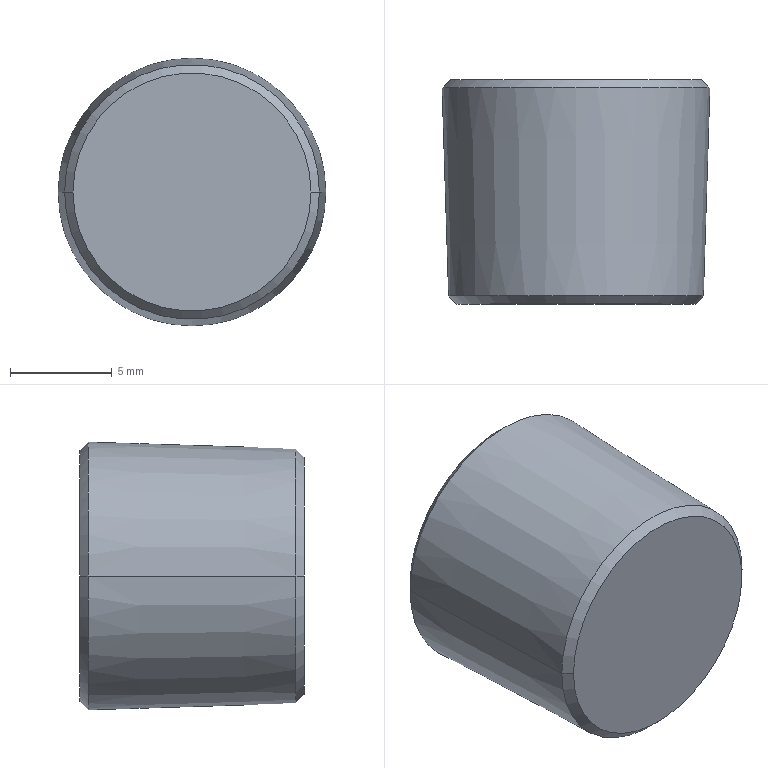Part | Creo | 1 solid | 15 faces | box 13.132 x 11 x 13.132 mm | volume 1254 mm3 | plane 9 | cone 6
STEP:
#1=CARTESIAN_POINT('',(89.838,199.,80.));
#2=VERTEX_POINT('',#1);
#3=CARTESIAN_POINT('',(78.162,199.,80.));
#4=VERTEX_POINT('',#3);
#5=CARTESIAN_POINT('',(84.,199.,80.));
#6=DIRECTION('',(0.,-1.,0.));
#7=DIRECTION('',(1.,0.,0.));
#8=AXIS2_PLACEMENT_3D('',#5,#6,#7);
#9=CIRCLE('',#8,5.838);
#10=EDGE_CURVE('',#2,#4,#9,.T.);
#11=ORIENTED_EDGE('',*,*,#10,.F.);
#12=CARTESIAN_POINT('',(84.,199.,80.));
#13=DIRECTION('',(0.,-1.,0.));
#14=DIRECTION('',(-1.,0.,0.));
#15=AXIS2_PLACEMENT_3D('',#12,#13,#14);
#16=CIRCLE('',#15,5.838);
#17=EDGE_CURVE('',#4,#2,#16,.T.);
#18=ORIENTED_EDGE('',*,*,#17,.F.);
#19=EDGE_LOOP('',(#11,#18));
#20=FACE_OUTER_BOUND('',#19,.F.);
#21=CARTESIAN_POINT('',(77.762,199.,80.));
#22=DIRECTION('',(0.,-1.,0.));
#23=DIRECTION('',(-1.,0.,0.));
#24=AXIS2_PLACEMENT_3D('',#21,#22,#23);
#25=PLANE('',#24);
#26=ADVANCED_FACE('',(#20),#25,.T.);
#27=ORIENTED_EDGE('',*,*,#10,.T.);
#28=CARTESIAN_POINT('',(77.75,199.4,80.));
#29=VERTEX_POINT('',#28);
#30=CARTESIAN_POINT('',(78.162,199.,80.));
#31=DIRECTION('',(-0.718,0.6961,0.));
#32=VECTOR('',#31,0.5744);
#33=LINE('',#30,#32);
#34=EDGE_CURVE('',#4,#29,#33,.T.);
#35=ORIENTED_EDGE('',*,*,#34,.T.);
#36=CARTESIAN_POINT('',(90.25,199.4,80.));
#37=VERTEX_POINT('',#36);
#38=CARTESIAN_POINT('',(84.,199.4,80.));
#39=DIRECTION('',(0.,-1.,0.));
#40=DIRECTION('',(1.,0.,0.));
#41=AXIS2_PLACEMENT_3D('',#38,#39,#40);
#42=CIRCLE('',#41,6.25);
#43=EDGE_CURVE('',#37,#29,#42,.T.);
#44=ORIENTED_EDGE('',*,*,#43,.F.);
#45=CARTESIAN_POINT('',(89.838,199.,80.));
#46=DIRECTION('',(0.718,0.6961,0.));
#47=VECTOR('',#46,0.5744);
#48=LINE('',#45,#47);
#49=EDGE_CURVE('',#2,#37,#48,.T.);
#50=ORIENTED_EDGE('',*,*,#49,.F.);
#51=EDGE_LOOP('',(#27,#35,#44,#50));
#52=FACE_OUTER_BOUND('',#51,.F.);
#53=CARTESIAN_POINT('',(84.,199.2,80.));
#54=DIRECTION('',(0.,1.,0.));
#55=DIRECTION('',(1.,0.,0.));
#56=AXIS2_PLACEMENT_3D('',#53,#54,#55);
#57=CONICAL_SURFACE('',#56,6.044,45.888);
#58=ADVANCED_FACE('',(#52),#57,.T.);
#59=ORIENTED_EDGE('',*,*,#17,.T.);
#60=ORIENTED_EDGE('',*,*,#49,.T.);
#61=CARTESIAN_POINT('',(84.,199.4,80.));
#62=DIRECTION('',(0.,-1.,0.));
#63=DIRECTION('',(-1.,0.,0.));
#64=AXIS2_PLACEMENT_3D('',#61,#62,#63);
#65=CIRCLE('',#64,6.25);
#66=EDGE_CURVE('',#29,#37,#65,.T.);
#67=ORIENTED_EDGE('',*,*,#66,.F.);
#68=ORIENTED_EDGE('',*,*,#34,.F.);
#69=EDGE_LOOP('',(#59,#60,#67,#68));
#70=FACE_OUTER_BOUND('',#69,.F.);
#71=CARTESIAN_POINT('',(84.,199.2,80.));
#72=DIRECTION('',(0.,1.,0.));
#73=DIRECTION('',(1.,0.,0.));
#74=AXIS2_PLACEMENT_3D('',#71,#72,#73);
#75=CONICAL_SURFACE('',#74,6.044,45.888);
#76=ADVANCED_FACE('',(#70),#75,.T.);
#77=ORIENTED_EDGE('',*,*,#66,.T.);
#78=CARTESIAN_POINT('',(90.566,209.6,80.));
#79=VERTEX_POINT('',#78);
#80=CARTESIAN_POINT('',(90.25,199.4,80.));
#81=DIRECTION('',(0.03097,0.9995,0.));
#82=VECTOR('',#81,10.205);
#83=LINE('',#80,#82);
#84=EDGE_CURVE('',#37,#79,#83,.T.);
#85=ORIENTED_EDGE('',*,*,#84,.T.);
#86=CARTESIAN_POINT('',(77.434,209.6,80.));
#87=VERTEX_POINT('',#86);
#88=CARTESIAN_POINT('',(84.,209.6,80.));
#89=DIRECTION('',(0.,1.,0.));
#90=DIRECTION('',(1.,0.,0.));
#91=AXIS2_PLACEMENT_3D('',#88,#89,#90);
#92=CIRCLE('',#91,6.566);
#93=EDGE_CURVE('',#79,#87,#92,.T.);
#94=ORIENTED_EDGE('',*,*,#93,.T.);
#95=CARTESIAN_POINT('',(77.75,199.4,80.));
#96=DIRECTION('',(-0.03097,0.9995,0.));
#97=VECTOR('',#96,10.205);
#98=LINE('',#95,#97);
#99=EDGE_CURVE('',#29,#87,#98,.T.);
#100=ORIENTED_EDGE('',*,*,#99,.F.);
#101=EDGE_LOOP('',(#77,#85,#94,#100));
#102=FACE_OUTER_BOUND('',#101,.F.);
#103=CARTESIAN_POINT('',(84.,204.5,80.));
#104=DIRECTION('',(0.,1.,0.));
#105=DIRECTION('',(1.,0.,0.));
#106=AXIS2_PLACEMENT_3D('',#103,#104,#105);
#107=CONICAL_SURFACE('',#106,6.408,1.775);
#108=ADVANCED_FACE('',(#102),#107,.T.);
#109=ORIENTED_EDGE('',*,*,#43,.T.);
#110=ORIENTED_EDGE('',*,*,#99,.T.);
#111=CARTESIAN_POINT('',(84.,209.6,80.));
#112=DIRECTION('',(0.,1.,0.));
#113=DIRECTION('',(-1.,0.,0.));
#114=AXIS2_PLACEMENT_3D('',#111,#112,#113);
#115=CIRCLE('',#114,6.566);
#116=EDGE_CURVE('',#87,#79,#115,.T.);
#117=ORIENTED_EDGE('',*,*,#116,.T.);
#118=ORIENTED_EDGE('',*,*,#84,.F.);
#119=EDGE_LOOP('',(#109,#110,#117,#118));
#120=FACE_OUTER_BOUND('',#119,.F.);
#121=CARTESIAN_POINT('',(84.,204.5,80.));
#122=DIRECTION('',(0.,1.,0.));
#123=DIRECTION('',(1.,0.,0.));
#124=AXIS2_PLACEMENT_3D('',#121,#122,#123);
#125=CONICAL_SURFACE('',#124,6.408,1.775);
#126=ADVANCED_FACE('',(#120),#125,.T.);
#127=ORIENTED_EDGE('',*,*,#116,.F.);
#128=CARTESIAN_POINT('',(77.821,210.,80.));
#129=VERTEX_POINT('',#128);
#130=CARTESIAN_POINT('',(77.821,210.,80.));
#131=DIRECTION('',(-0.6961,-0.718,0.));
#132=VECTOR('',#131,0.5569);
#133=LINE('',#130,#132);
#134=EDGE_CURVE('',#129,#87,#133,.T.);
#135=ORIENTED_EDGE('',*,*,#134,.F.);
#136=CARTESIAN_POINT('',(90.178,210.,80.));
#137=VERTEX_POINT('',#136);
#138=CARTESIAN_POINT('',(84.,210.,80.));
#139=DIRECTION('',(0.,1.,0.));
#140=DIRECTION('',(-1.,0.,0.));
#141=AXIS2_PLACEMENT_3D('',#138,#139,#140);
#142=CIRCLE('',#141,6.178);
#143=EDGE_CURVE('',#129,#137,#142,.T.);
#144=ORIENTED_EDGE('',*,*,#143,.T.);
#145=CARTESIAN_POINT('',(90.178,210.,80.));
#146=DIRECTION('',(0.6961,-0.718,0.));
#147=VECTOR('',#146,0.5569);
#148=LINE('',#145,#147);
#149=EDGE_CURVE('',#137,#79,#148,.T.);
#150=ORIENTED_EDGE('',*,*,#149,.T.);
#151=EDGE_LOOP('',(#127,#135,#144,#150));
#152=FACE_OUTER_BOUND('',#151,.F.);
#153=CARTESIAN_POINT('',(84.,209.8,80.));
#154=DIRECTION('',(0.,-1.,0.));
#155=DIRECTION('',(-1.,0.,0.));
#156=AXIS2_PLACEMENT_3D('',#153,#154,#155);
#157=CONICAL_SURFACE('',#156,6.372,44.112);
#158=ADVANCED_FACE('',(#152),#157,.T.);
#159=ORIENTED_EDGE('',*,*,#93,.F.);
#160=ORIENTED_EDGE('',*,*,#149,.F.);
#161=CARTESIAN_POINT('',(84.,210.,80.));
#162=DIRECTION('',(0.,1.,0.));
#163=DIRECTION('',(1.,0.,0.));
#164=AXIS2_PLACEMENT_3D('',#161,#162,#163);
#165=CIRCLE('',#164,6.178);
#166=EDGE_CURVE('',#137,#129,#165,.T.);
#167=ORIENTED_EDGE('',*,*,#166,.T.);
#168=ORIENTED_EDGE('',*,*,#134,.T.);
#169=EDGE_LOOP('',(#159,#160,#167,#168));
#170=FACE_OUTER_BOUND('',#169,.F.);
#171=CARTESIAN_POINT('',(84.,209.8,80.));
#172=DIRECTION('',(0.,-1.,0.));
#173=DIRECTION('',(-1.,0.,0.));
#174=AXIS2_PLACEMENT_3D('',#171,#172,#173);
#175=CONICAL_SURFACE('',#174,6.372,44.112);
#176=ADVANCED_FACE('',(#170),#175,.T.);
#177=ORIENTED_EDGE('',*,*,#143,.F.);
#178=ORIENTED_EDGE('',*,*,#166,.F.);
#179=EDGE_LOOP('',(#177,#178));
#180=FACE_OUTER_BOUND('',#179,.F.);
#181=CARTESIAN_POINT('',(85.75,210.,76.969));
#182=VERTEX_POINT('',#181);
#183=CARTESIAN_POINT('',(87.5,210.,80.));
#184=VERTEX_POINT('',#183);
#185=CARTESIAN_POINT('',(85.75,210.,76.969));
#186=DIRECTION('',(0.5,0.,0.866));
#187=VECTOR('',#186,3.5);
#188=LINE('',#185,#187);
#189=EDGE_CURVE('',#182,#184,#188,.T.);
#190=ORIENTED_EDGE('',*,*,#189,.F.);
#191=CARTESIAN_POINT('',(82.25,210.,76.969));
#192=VERTEX_POINT('',#191);
#193=CARTESIAN_POINT('',(82.25,210.,76.969));
#194=DIRECTION('',(1.,0.,0.));
#195=VECTOR('',#194,3.5);
#196=LINE('',#193,#195);
#197=EDGE_CURVE('',#192,#182,#196,.T.);
#198=ORIENTED_EDGE('',*,*,#197,.F.);
#199=CARTESIAN_POINT('',(80.5,210.,80.));
#200=VERTEX_POINT('',#199);
#201=CARTESIAN_POINT('',(80.5,210.,80.));
#202=DIRECTION('',(0.5,0.,-0.866));
#203=VECTOR('',#202,3.5);
#204=LINE('',#201,#203);
#205=EDGE_CURVE('',#200,#192,#204,.T.);
#206=ORIENTED_EDGE('',*,*,#205,.F.);
#207=CARTESIAN_POINT('',(82.25,210.,83.031));
#208=VERTEX_POINT('',#207);
#209=CARTESIAN_POINT('',(82.25,210.,83.031));
#210=DIRECTION('',(-0.5,0.,-0.866));
#211=VECTOR('',#210,3.5);
#212=LINE('',#209,#211);
#213=EDGE_CURVE('',#208,#200,#212,.T.);
#214=ORIENTED_EDGE('',*,*,#213,.F.);
#215=CARTESIAN_POINT('',(85.75,210.,83.031));
#216=VERTEX_POINT('',#215);
#217=CARTESIAN_POINT('',(85.75,210.,83.031));
#218=DIRECTION('',(-1.,0.,0.));
#219=VECTOR('',#218,3.5);
#220=LINE('',#217,#219);
#221=EDGE_CURVE('',#216,#208,#220,.T.);
#222=ORIENTED_EDGE('',*,*,#221,.F.);
#223=CARTESIAN_POINT('',(87.5,210.,80.));
#224=DIRECTION('',(-0.5,0.,0.866));
#225=VECTOR('',#224,3.5);
#226=LINE('',#223,#225);
#227=EDGE_CURVE('',#184,#216,#226,.T.);
#228=ORIENTED_EDGE('',*,*,#227,.F.);
#229=EDGE_LOOP('',(#190,#198,#206,#214,#222,#228));
#230=FACE_BOUND('',#229,.F.);
#231=CARTESIAN_POINT('',(84.,210.,80.));
#232=DIRECTION('',(0.,1.,0.));
#233=DIRECTION('',(1.,0.,0.));
#234=AXIS2_PLACEMENT_3D('',#231,#232,#233);
#235=PLANE('',#234);
#236=ADVANCED_FACE('',(#180,#230),#235,.T.);
#237=ORIENTED_EDGE('',*,*,#189,.T.);
#238=CARTESIAN_POINT('',(87.5,205.,80.));
#239=VERTEX_POINT('',#238);
#240=CARTESIAN_POINT('',(87.5,205.,80.));
#241=DIRECTION('',(0.,1.,0.));
#242=VECTOR('',#241,5.);
#243=LINE('',#240,#242);
#244=EDGE_CURVE('',#239,#184,#243,.T.);
#245=ORIENTED_EDGE('',*,*,#244,.F.);
#246=CARTESIAN_POINT('',(85.75,205.,76.969));
#247=VERTEX_POINT('',#246);
#248=CARTESIAN_POINT('',(87.5,205.,80.));
#249=DIRECTION('',(-0.5,0.,-0.866));
#250=VECTOR('',#249,3.5);
#251=LINE('',#248,#250);
#252=EDGE_CURVE('',#239,#247,#251,.T.);
#253=ORIENTED_EDGE('',*,*,#252,.T.);
#254=CARTESIAN_POINT('',(85.75,205.,76.969));
#255=DIRECTION('',(0.,1.,0.));
#256=VECTOR('',#255,5.);
#257=LINE('',#254,#256);
#258=EDGE_CURVE('',#247,#182,#257,.T.);
#259=ORIENTED_EDGE('',*,*,#258,.T.);
#260=EDGE_LOOP('',(#237,#245,#253,#259));
#261=FACE_OUTER_BOUND('',#260,.F.);
#262=CARTESIAN_POINT('',(87.5,205.,80.));
#263=DIRECTION('',(0.866,0.,-0.5));
#264=DIRECTION('',(0.5,0.,0.866));
#265=AXIS2_PLACEMENT_3D('',#262,#263,#264);
#266=PLANE('',#265);
#267=ADVANCED_FACE('',(#261),#266,.F.);
#268=ORIENTED_EDGE('',*,*,#227,.T.);
#269=CARTESIAN_POINT('',(85.75,205.,83.031));
#270=VERTEX_POINT('',#269);
#271=CARTESIAN_POINT('',(85.75,205.,83.031));
#272=DIRECTION('',(0.,1.,0.));
#273=VECTOR('',#272,5.);
#274=LINE('',#271,#273);
#275=EDGE_CURVE('',#270,#216,#274,.T.);
#276=ORIENTED_EDGE('',*,*,#275,.F.);
#277=CARTESIAN_POINT('',(85.75,205.,83.031));
#278=DIRECTION('',(0.5,0.,-0.866));
#279=VECTOR('',#278,3.5);
#280=LINE('',#277,#279);
#281=EDGE_CURVE('',#270,#239,#280,.T.);
#282=ORIENTED_EDGE('',*,*,#281,.T.);
#283=ORIENTED_EDGE('',*,*,#244,.T.);
#284=EDGE_LOOP('',(#268,#276,#282,#283));
#285=FACE_OUTER_BOUND('',#284,.F.);
#286=CARTESIAN_POINT('',(85.75,205.,83.031));
#287=DIRECTION('',(0.866,0.,0.5));
#288=DIRECTION('',(-0.5,0.,0.866));
#289=AXIS2_PLACEMENT_3D('',#286,#287,#288);
#290=PLANE('',#289);
#291=ADVANCED_FACE('',(#285),#290,.F.);
#292=ORIENTED_EDGE('',*,*,#221,.T.);
#293=CARTESIAN_POINT('',(82.25,205.,83.031));
#294=VERTEX_POINT('',#293);
#295=CARTESIAN_POINT('',(82.25,205.,83.031));
#296=DIRECTION('',(0.,1.,0.));
#297=VECTOR('',#296,5.);
#298=LINE('',#295,#297);
#299=EDGE_CURVE('',#294,#208,#298,.T.);
#300=ORIENTED_EDGE('',*,*,#299,.F.);
#301=CARTESIAN_POINT('',(82.25,205.,83.031));
#302=DIRECTION('',(1.,0.,0.));
#303=VECTOR('',#302,3.5);
#304=LINE('',#301,#303);
#305=EDGE_CURVE('',#294,#270,#304,.T.);
#306=ORIENTED_EDGE('',*,*,#305,.T.);
#307=ORIENTED_EDGE('',*,*,#275,.T.);
#308=EDGE_LOOP('',(#292,#300,#306,#307));
#309=FACE_OUTER_BOUND('',#308,.F.);
#310=CARTESIAN_POINT('',(82.25,205.,83.031));
#311=DIRECTION('',(0.,0.,1.));
#312=DIRECTION('',(-1.,0.,0.));
#313=AXIS2_PLACEMENT_3D('',#310,#311,#312);
#314=PLANE('',#313);
#315=ADVANCED_FACE('',(#309),#314,.F.);
#316=ORIENTED_EDGE('',*,*,#213,.T.);
#317=CARTESIAN_POINT('',(80.5,205.,80.));
#318=VERTEX_POINT('',#317);
#319=CARTESIAN_POINT('',(80.5,205.,80.));
#320=DIRECTION('',(0.,1.,0.));
#321=VECTOR('',#320,5.);
#322=LINE('',#319,#321);
#323=EDGE_CURVE('',#318,#200,#322,.T.);
#324=ORIENTED_EDGE('',*,*,#323,.F.);
#325=CARTESIAN_POINT('',(80.5,205.,80.));
#326=DIRECTION('',(0.5,0.,0.866));
#327=VECTOR('',#326,3.5);
#328=LINE('',#325,#327);
#329=EDGE_CURVE('',#318,#294,#328,.T.);
#330=ORIENTED_EDGE('',*,*,#329,.T.);
#331=ORIENTED_EDGE('',*,*,#299,.T.);
#332=EDGE_LOOP('',(#316,#324,#330,#331));
#333=FACE_OUTER_BOUND('',#332,.F.);
#334=CARTESIAN_POINT('',(80.5,205.,80.));
#335=DIRECTION('',(-0.866,0.,0.5));
#336=DIRECTION('',(-0.5,0.,-0.866));
#337=AXIS2_PLACEMENT_3D('',#334,#335,#336);
#338=PLANE('',#337);
#339=ADVANCED_FACE('',(#333),#338,.F.);
#340=ORIENTED_EDGE('',*,*,#205,.T.);
#341=CARTESIAN_POINT('',(82.25,205.,76.969));
#342=VERTEX_POINT('',#341);
#343=CARTESIAN_POINT('',(82.25,205.,76.969));
#344=DIRECTION('',(0.,1.,0.));
#345=VECTOR('',#344,5.);
#346=LINE('',#343,#345);
#347=EDGE_CURVE('',#342,#192,#346,.T.);
#348=ORIENTED_EDGE('',*,*,#347,.F.);
#349=CARTESIAN_POINT('',(82.25,205.,76.969));
#350=DIRECTION('',(-0.5,0.,0.866));
#351=VECTOR('',#350,3.5);
#352=LINE('',#349,#351);
#353=EDGE_CURVE('',#342,#318,#352,.T.);
#354=ORIENTED_EDGE('',*,*,#353,.T.);
#355=ORIENTED_EDGE('',*,*,#323,.T.);
#356=EDGE_LOOP('',(#340,#348,#354,#355));
#357=FACE_OUTER_BOUND('',#356,.F.);
#358=CARTESIAN_POINT('',(82.25,205.,76.969));
#359=DIRECTION('',(-0.866,0.,-0.5));
#360=DIRECTION('',(0.5,0.,-0.866));
#361=AXIS2_PLACEMENT_3D('',#358,#359,#360);
#362=PLANE('',#361);
#363=ADVANCED_FACE('',(#357),#362,.F.);
#364=ORIENTED_EDGE('',*,*,#197,.T.);
#365=ORIENTED_EDGE('',*,*,#258,.F.);
#366=CARTESIAN_POINT('',(85.75,205.,76.969));
#367=DIRECTION('',(-1.,0.,0.));
#368=VECTOR('',#367,3.5);
#369=LINE('',#366,#368);
#370=EDGE_CURVE('',#247,#342,#369,.T.);
#371=ORIENTED_EDGE('',*,*,#370,.T.);
#372=ORIENTED_EDGE('',*,*,#347,.T.);
#373=EDGE_LOOP('',(#364,#365,#371,#372));
#374=FACE_OUTER_BOUND('',#373,.F.);
#375=CARTESIAN_POINT('',(85.75,205.,76.969));
#376=DIRECTION('',(0.,0.,-1.));
#377=DIRECTION('',(1.,0.,0.));
#378=AXIS2_PLACEMENT_3D('',#375,#376,#377);
#379=PLANE('',#378);
#380=ADVANCED_FACE('',(#374),#379,.F.);
#381=ORIENTED_EDGE('',*,*,#252,.F.);
#382=ORIENTED_EDGE('',*,*,#281,.F.);
#383=ORIENTED_EDGE('',*,*,#305,.F.);
#384=ORIENTED_EDGE('',*,*,#329,.F.);
#385=ORIENTED_EDGE('',*,*,#353,.F.);
#386=ORIENTED_EDGE('',*,*,#370,.F.);
#387=EDGE_LOOP('',(#381,#382,#383,#384,#385,#386));
#388=FACE_OUTER_BOUND('',#387,.F.);
#389=CARTESIAN_POINT('',(84.,205.,80.));
#390=DIRECTION('',(0.,1.,0.));
#391=DIRECTION('',(1.,0.,0.));
#392=AXIS2_PLACEMENT_3D('',#389,#390,#391);
#393=PLANE('',#392);
#394=ADVANCED_FACE('',(#388),#393,.T.);
#395=CLOSED_SHELL('',(#26,#58,#76,#108,#126,#158,#176,#236,#267,#291,#315,#339,#363,#380,#394));
#396=MANIFOLD_SOLID_BREP('',#395);
#397=(LENGTH_UNIT()NAMED_UNIT(*)SI_UNIT(.MILLI.,.METRE.));
#398=UNCERTAINTY_MEASURE_WITH_UNIT(LENGTH_MEASURE(0.002158),#397,'','');
#399=(NAMED_UNIT(*)PLANE_ANGLE_UNIT()SI_UNIT($,.RADIAN.));
#400=PLANE_ANGLE_MEASURE_WITH_UNIT(PLANE_ANGLE_MEASURE(0.01745),#399);
#401=(CONVERSION_BASED_UNIT('DEGREE',#400)NAMED_UNIT(*)PLANE_ANGLE_UNIT());
#402=(NAMED_UNIT(*)SI_UNIT($,.STERADIAN.)SOLID_ANGLE_UNIT());
#403=(GEOMETRIC_REPRESENTATION_CONTEXT(3)GLOBAL_UNCERTAINTY_ASSIGNED_CONTEXT((#398))GLOBAL_UNIT_ASSIGNED_CONTEXT((#397,#401,#402))REPRESENTATION_CONTEXT('',''));
#404=ADVANCED_BREP_SHAPE_REPRESENTATION('',(#396),#403);